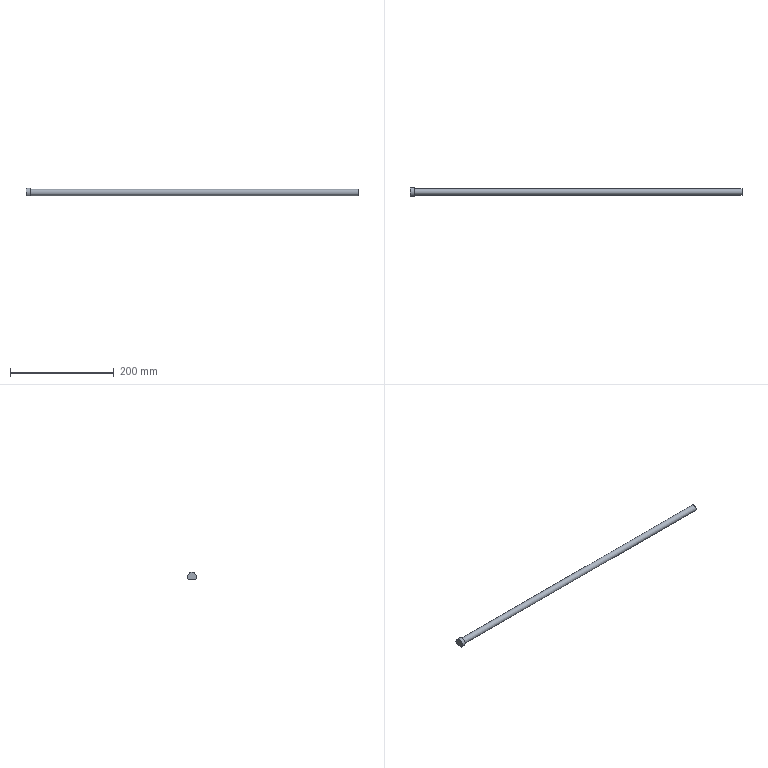Part | STEP file | solid 34 | 1 solid | 6 faces | box 640 x 17 x 15 mm | volume 73173 mm3 | plane 4 | cylinder 2 | commonest cylinder face diameters 12 x1 17 x1